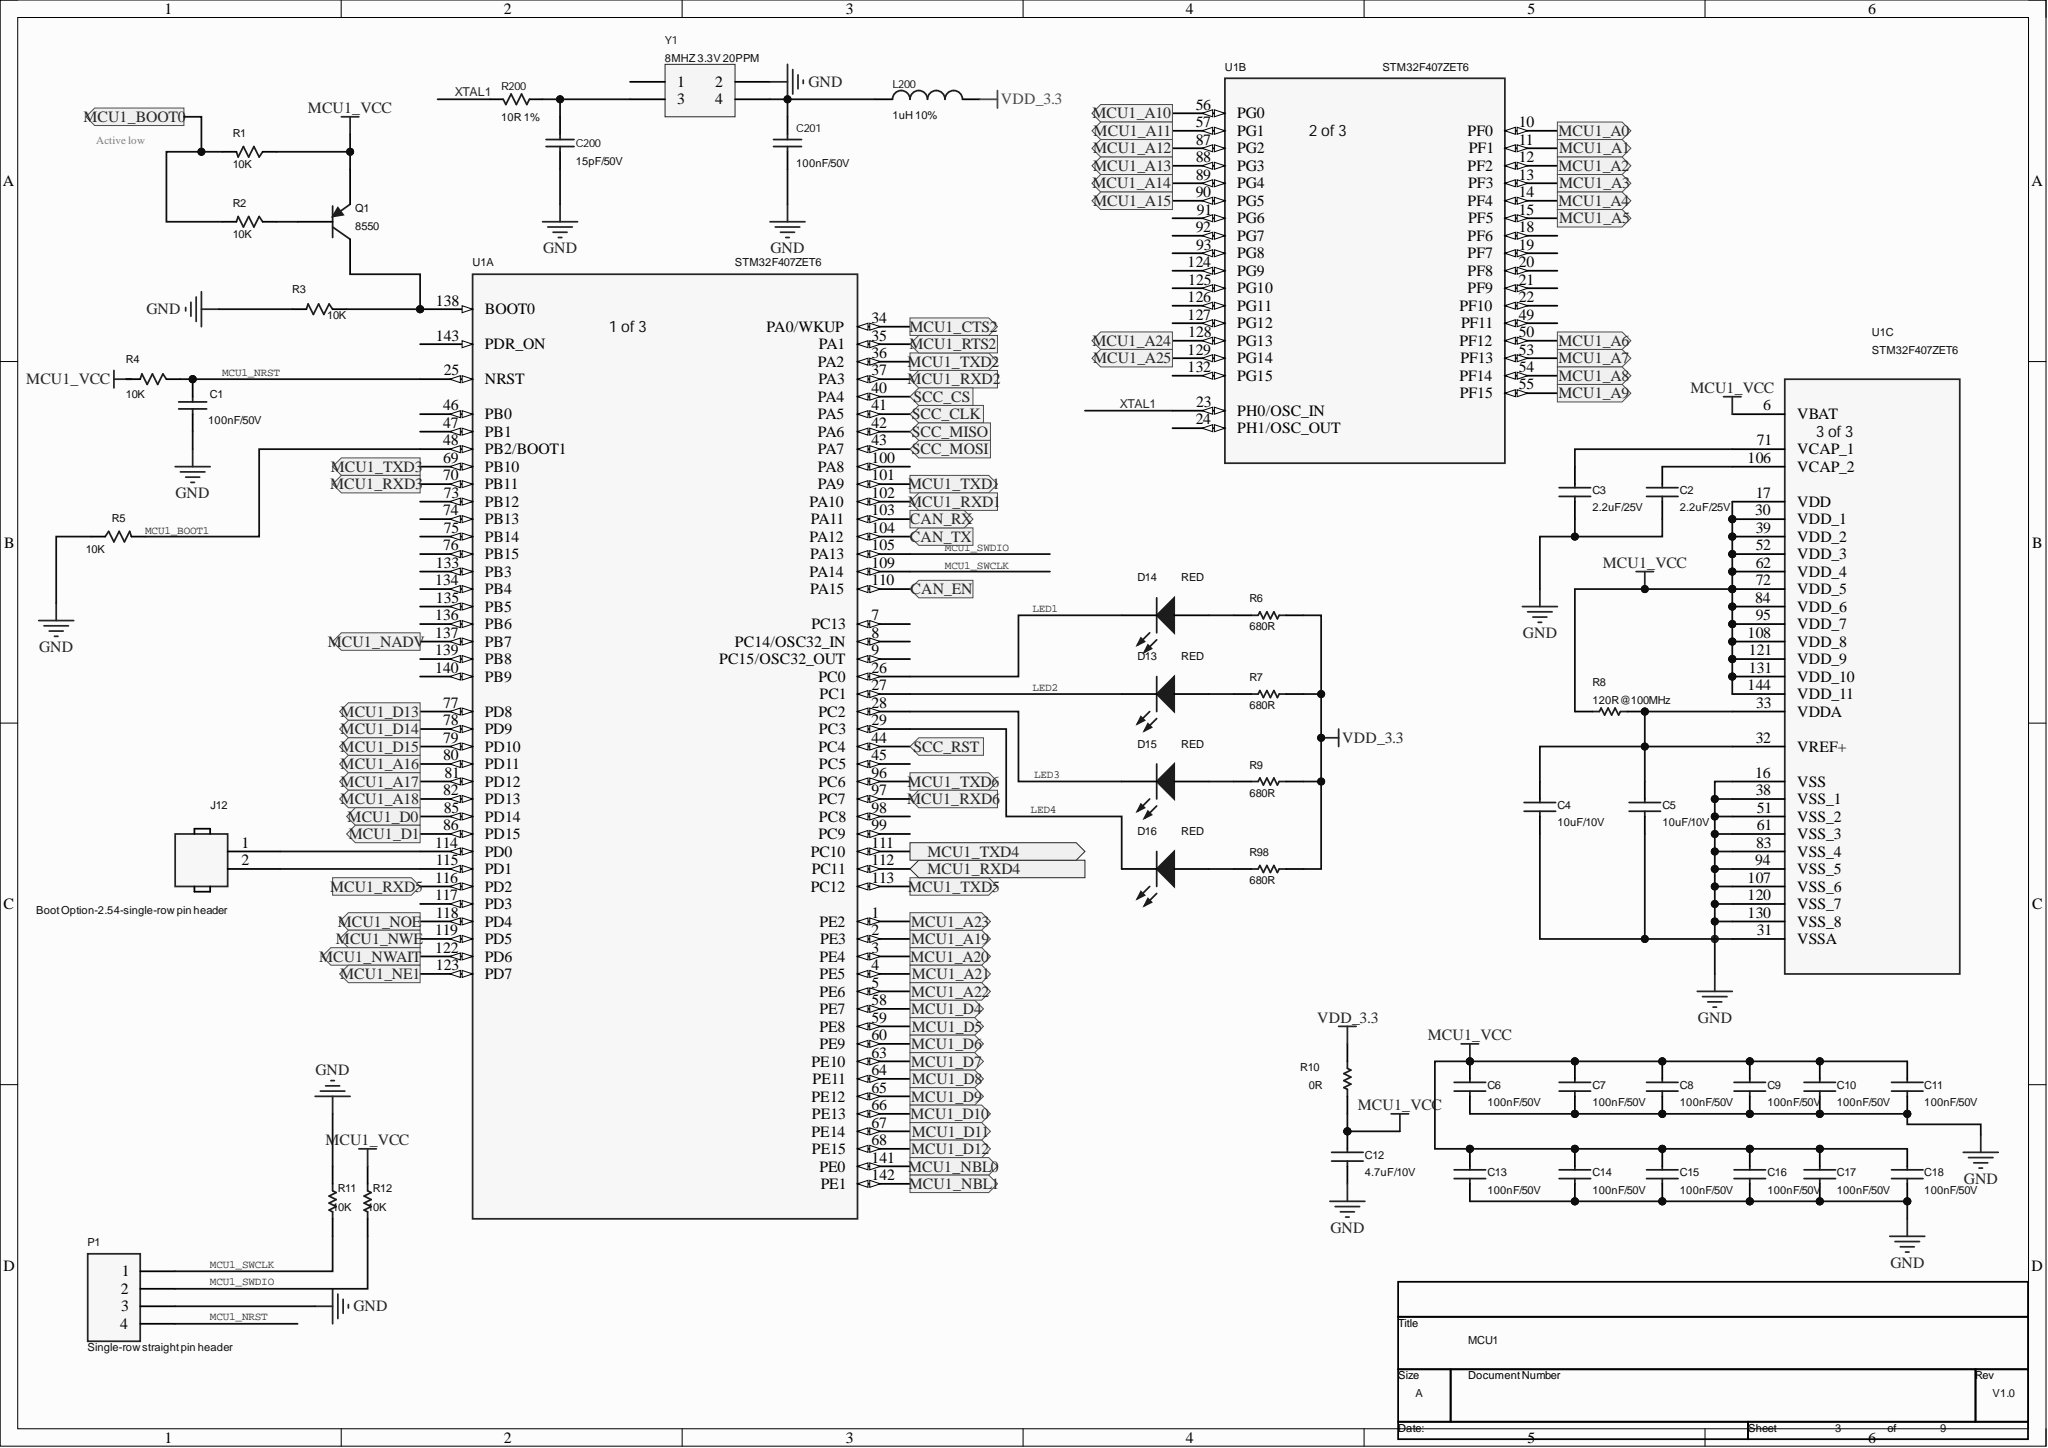Circuit board | Altium Designer | 313 parts | 216 nets | one sheet of the schematic
Parts on this sheet (reference | value | footprint):
C1 | 100nF/50V | 0603
C2 | 2.2uF/25V | C0603
C3 | 2.2uF/25V | C0603
C4 | 10uF/10V | C0603
C5 | 10uF/10V | C0603
C6 | 100nF/50V | C0603
C7 | 100nF/50V | C0603
C8 | 100nF/50V | C0603
C9 | 100nF/50V | C0603
C10 | 100nF/50V | C0603
C11 | 100nF/50V | C0603
C12 | 4.7uF/10V | C0805
C13 | 100nF/50V | C0603
C14 | 100nF/50V | C0603
C15 | 100nF/50V | C0603
C16 | 100nF/50V | C0603
C17 | 100nF/50V | C0603
C18 | 100nF/50V | C0603
C200 | 15pF/50V | C0603
C201 | 100nF/50V | C0603
D13 | RED | LED_0805
D14 | RED | LED_0805
D15 | RED | LED_0805
D16 | RED | LED_0805
J12 | Boot Option-2.54-single-row pin header | HDR_1X2_254
L200 | 1uH 10% | SMD_L6.0-W6.0
P1 | Single-row straight pin header | HDR1X4
Q1 | 8550 | SOT-23-SS8550
R1 | 10K | 0603
R2 | 10K | 0603
R3 | 10K | 0603
R4 | 10K | 0603
R5 | 10K | 0603
R6 | NA | 0603
R7 | NA | 0603
R8 | 120R@100MHz | 0603
R9 | NA | 0603
R10 | 0R | 0603
R11 | 10K | 0603
R12 | 10K | 0603
R98 | NA | 0603
R200 | 10R 1% | R0805
U1 | STM32F407ZET6 | LQFP144-20x20mm
Y1 | 8MHZ 3.3V 20PPM | XTAL 5.7X7.0-SM - duplicate
Nets of these parts (net: part-pin ...):
XTAL1: R200-1 U1-23
VDD_3.3: L200-2 R6-1 R7-1 R9-1 R10-1 R98-1
NetQ1_3: Q1-3 R3-2 U1-138
NetQ1_1: Q1-1 R2-1
NetP3_11: R1-1 R2-2
NetJ12_2: J12-2 U1-115
NetJ12_1: J12-1 U1-114
NetD16_1: D16-1 R98-2
NetD15_1: D15-1 R9-2
NetD14_1: D14-1 R6-2
NetD13_1: D13-1 R7-2
NetC201_1: C201-1 L200-1 Y1-4
NetC200_2: C200-2 R200-2 Y1-3
NetC4_1: C4-1 C5-1 R8-2 U1-32 U1-33
NetC3_1: C3-1 U1-71
NetC2_1: C2-1 U1-106
MCU1_VCC: C6-1 C7-1 C8-1 C9-1 C10-1 C11-1 C12-1 C13-1 C14-1 C15-1 C16-1 C17-1 C18-1 Q1-2 R1-2 R4-2 R8-1 R10-2 R12-2 U1-6 U1-17 U1-30 U1-39 U1-52 U1-62 U1-72 U1-84 U1-95 U1-108 U1-121 U1-131 U1-144
MCU1_SWDIO: P1-2 R12-1 U1-105
MCU1_SWCLK: P1-1 R11-1 U1-109
MCU1_NRST: C1-2 P1-4 R4-1 U1-25
MCU1_BOOT1: R5-2 U1-48
LED4: D16-2 U1-29
LED3: D15-2 U1-28
LED2: D13-2 U1-27
LED1: D14-2 U1-26
GND: C1-1 C2-2 C3-2 C4-2 C5-2 C6-2 C7-2 C8-2 C9-2 C10-2 C11-2 C12-2 C13-2 C14-2 C15-2 C16-2 C17-2 C18-2 C200-1 C201-2 P1-3 R3-1 R5-1 R11-2 Y1-2 U1-16 U1-31 U1-38 U1-51 U1-61 U1-83 U1-94 U1-107 U1-120 U1-130